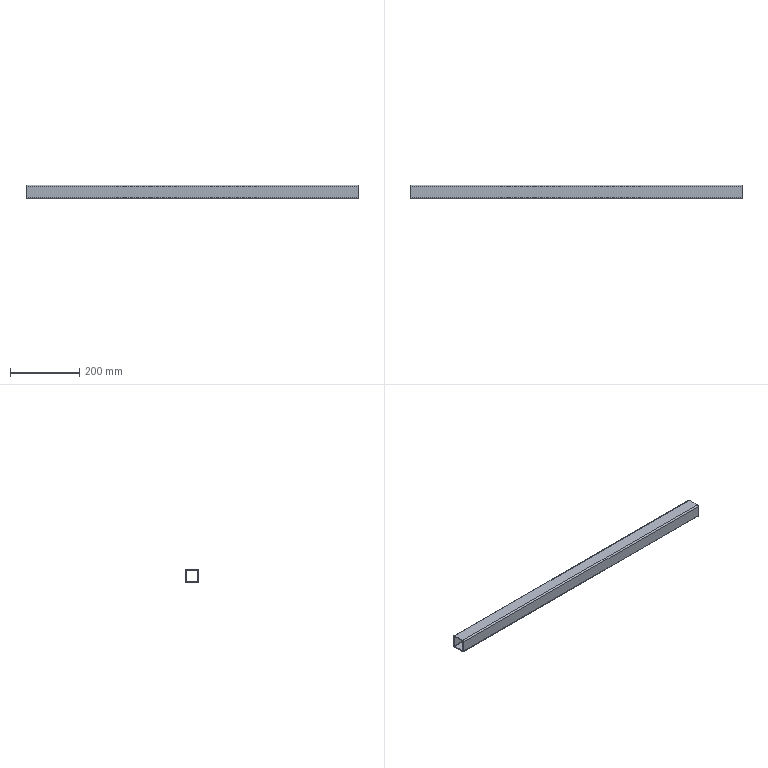Part | 1 solid | 22 faces | box 956 x 40 x 40 mm | volume 410269 mm3 | cylinder 12 | plane 10 | commonest cylinder face diameters 2 x4 8 x4 20 x4
STEP:
#1=CARTESIAN_POINT('',(40.,0.,-17.));
#2=VERTEX_POINT('',#1);
#3=CARTESIAN_POINT('',(60.,0.,-17.));
#4=VERTEX_POINT('',#3);
#5=CARTESIAN_POINT('',(50.,0.,-17.));
#6=DIRECTION('',(0.,0.,1.));
#7=DIRECTION('',(1.,0.,0.));
#8=AXIS2_PLACEMENT_3D('',#5,#6,#7);
#9=CIRCLE('',#8,10.);
#10=EDGE_CURVE('',#2,#4,#9,.T.);
#11=ORIENTED_EDGE('',*,*,#10,.T.);
#12=CARTESIAN_POINT('',(60.,0.,-20.));
#13=VERTEX_POINT('',#12);
#14=CARTESIAN_POINT('',(60.,0.,-10.));
#15=DIRECTION('',(0.,0.,-1.));
#16=VECTOR('',#15,1000.);
#17=LINE('',#14,#16);
#18=EDGE_CURVE('',#4,#13,#17,.T.);
#19=ORIENTED_EDGE('',*,*,#18,.T.);
#20=CARTESIAN_POINT('',(40.,0.,-20.));
#21=VERTEX_POINT('',#20);
#22=CARTESIAN_POINT('',(50.,0.,-20.));
#23=DIRECTION('',(0.,0.,-1.));
#24=DIRECTION('',(-1.,0.,0.));
#25=AXIS2_PLACEMENT_3D('',#22,#23,#24);
#26=CIRCLE('',#25,10.);
#27=EDGE_CURVE('',#13,#21,#26,.T.);
#28=ORIENTED_EDGE('',*,*,#27,.T.);
#29=CARTESIAN_POINT('',(40.,0.,-10.));
#30=DIRECTION('',(0.,0.,-1.));
#31=VECTOR('',#30,1000.);
#32=LINE('',#29,#31);
#33=EDGE_CURVE('',#2,#21,#32,.T.);
#34=ORIENTED_EDGE('',*,*,#33,.F.);
#35=EDGE_LOOP('',(#11,#19,#28,#34));
#36=FACE_OUTER_BOUND('',#35,.T.);
#37=CARTESIAN_POINT('',(50.,0.,-10.));
#38=DIRECTION('',(0.,0.,-1.));
#39=DIRECTION('',(-1.,0.,0.));
#40=AXIS2_PLACEMENT_3D('',#37,#38,#39);
#41=CYLINDRICAL_SURFACE('',#40,10.);
#42=ADVANCED_FACE('',(#36),#41,.F.);
#43=CARTESIAN_POINT('',(921.,0.,-17.));
#44=VERTEX_POINT('',#43);
#45=CARTESIAN_POINT('',(941.,0.,-17.));
#46=VERTEX_POINT('',#45);
#47=CARTESIAN_POINT('',(931.,0.,-17.));
#48=DIRECTION('',(0.,0.,1.));
#49=DIRECTION('',(1.,0.,0.));
#50=AXIS2_PLACEMENT_3D('',#47,#48,#49);
#51=CIRCLE('',#50,10.);
#52=EDGE_CURVE('',#44,#46,#51,.T.);
#53=ORIENTED_EDGE('',*,*,#52,.T.);
#54=CARTESIAN_POINT('',(941.,0.,-20.));
#55=VERTEX_POINT('',#54);
#56=CARTESIAN_POINT('',(941.,0.,-10.));
#57=DIRECTION('',(0.,0.,-1.));
#58=VECTOR('',#57,1000.);
#59=LINE('',#56,#58);
#60=EDGE_CURVE('',#46,#55,#59,.T.);
#61=ORIENTED_EDGE('',*,*,#60,.T.);
#62=CARTESIAN_POINT('',(921.,0.,-20.));
#63=VERTEX_POINT('',#62);
#64=CARTESIAN_POINT('',(931.,0.,-20.));
#65=DIRECTION('',(0.,0.,-1.));
#66=DIRECTION('',(-1.,0.,0.));
#67=AXIS2_PLACEMENT_3D('',#64,#65,#66);
#68=CIRCLE('',#67,10.);
#69=EDGE_CURVE('',#55,#63,#68,.T.);
#70=ORIENTED_EDGE('',*,*,#69,.T.);
#71=CARTESIAN_POINT('',(921.,0.,-10.));
#72=DIRECTION('',(0.,0.,-1.));
#73=VECTOR('',#72,1000.);
#74=LINE('',#71,#73);
#75=EDGE_CURVE('',#44,#63,#74,.T.);
#76=ORIENTED_EDGE('',*,*,#75,.F.);
#77=EDGE_LOOP('',(#53,#61,#70,#76));
#78=FACE_OUTER_BOUND('',#77,.T.);
#79=CARTESIAN_POINT('',(931.,0.,-10.));
#80=DIRECTION('',(0.,0.,-1.));
#81=DIRECTION('',(-1.,0.,0.));
#82=AXIS2_PLACEMENT_3D('',#79,#80,#81);
#83=CYLINDRICAL_SURFACE('',#82,10.);
#84=ADVANCED_FACE('',(#78),#83,.F.);
#85=CARTESIAN_POINT('',(0.,20.,16.));
#86=VERTEX_POINT('',#85);
#87=CARTESIAN_POINT('',(0.,16.,20.));
#88=VERTEX_POINT('',#87);
#89=CARTESIAN_POINT('',(0.,16.,16.));
#90=DIRECTION('',(1.,0.,0.));
#91=DIRECTION('',(0.,0.,-1.));
#92=AXIS2_PLACEMENT_3D('',#89,#90,#91);
#93=CIRCLE('',#92,4.);
#94=EDGE_CURVE('',#86,#88,#93,.T.);
#95=ORIENTED_EDGE('',*,*,#94,.T.);
#96=CARTESIAN_POINT('',(956.,16.,20.));
#97=VERTEX_POINT('',#96);
#98=CARTESIAN_POINT('',(956.,16.,20.));
#99=DIRECTION('',(-1.,0.,0.));
#100=VECTOR('',#99,1000.);
#101=LINE('',#98,#100);
#102=EDGE_CURVE('',#97,#88,#101,.T.);
#103=ORIENTED_EDGE('',*,*,#102,.F.);
#104=CARTESIAN_POINT('',(956.,20.,16.));
#105=VERTEX_POINT('',#104);
#106=CARTESIAN_POINT('',(956.,16.,16.));
#107=DIRECTION('',(1.,0.,0.));
#108=DIRECTION('',(0.,0.,-1.));
#109=AXIS2_PLACEMENT_3D('',#106,#107,#108);
#110=CIRCLE('',#109,4.);
#111=EDGE_CURVE('',#105,#97,#110,.T.);
#112=ORIENTED_EDGE('',*,*,#111,.F.);
#113=CARTESIAN_POINT('',(956.,20.,16.));
#114=DIRECTION('',(-1.,0.,0.));
#115=VECTOR('',#114,1000.);
#116=LINE('',#113,#115);
#117=EDGE_CURVE('',#105,#86,#116,.T.);
#118=ORIENTED_EDGE('',*,*,#117,.T.);
#119=EDGE_LOOP('',(#95,#103,#112,#118));
#120=FACE_OUTER_BOUND('',#119,.T.);
#121=CARTESIAN_POINT('',(956.,16.,16.));
#122=DIRECTION('',(-1.,0.,0.));
#123=DIRECTION('',(0.,0.,1.));
#124=AXIS2_PLACEMENT_3D('',#121,#122,#123);
#125=CYLINDRICAL_SURFACE('',#124,4.);
#126=ADVANCED_FACE('',(#120),#125,.T.);
#127=CARTESIAN_POINT('',(0.,-16.,20.));
#128=VERTEX_POINT('',#127);
#129=CARTESIAN_POINT('',(0.,16.,20.));
#130=DIRECTION('',(0.,-1.,0.));
#131=VECTOR('',#130,1000.);
#132=LINE('',#129,#131);
#133=EDGE_CURVE('',#88,#128,#132,.T.);
#134=ORIENTED_EDGE('',*,*,#133,.T.);
#135=CARTESIAN_POINT('',(956.,-16.,20.));
#136=VERTEX_POINT('',#135);
#137=CARTESIAN_POINT('',(956.,-16.,20.));
#138=DIRECTION('',(-1.,0.,0.));
#139=VECTOR('',#138,1000.);
#140=LINE('',#137,#139);
#141=EDGE_CURVE('',#136,#128,#140,.T.);
#142=ORIENTED_EDGE('',*,*,#141,.F.);
#143=CARTESIAN_POINT('',(956.,16.,20.));
#144=DIRECTION('',(0.,-1.,0.));
#145=VECTOR('',#144,1000.);
#146=LINE('',#143,#145);
#147=EDGE_CURVE('',#97,#136,#146,.T.);
#148=ORIENTED_EDGE('',*,*,#147,.F.);
#149=ORIENTED_EDGE('',*,*,#102,.T.);
#150=EDGE_LOOP('',(#134,#142,#148,#149));
#151=FACE_OUTER_BOUND('',#150,.T.);
#152=CARTESIAN_POINT('',(956.,16.,20.));
#153=DIRECTION('',(0.,0.,-1.));
#154=DIRECTION('',(-1.,0.,0.));
#155=AXIS2_PLACEMENT_3D('',#152,#153,#154);
#156=PLANE('',#155);
#157=ADVANCED_FACE('',(#151),#156,.F.);
#158=CARTESIAN_POINT('',(0.,-20.,16.));
#159=VERTEX_POINT('',#158);
#160=CARTESIAN_POINT('',(0.,-16.,16.));
#161=DIRECTION('',(1.,0.,0.));
#162=DIRECTION('',(0.,0.,-1.));
#163=AXIS2_PLACEMENT_3D('',#160,#161,#162);
#164=CIRCLE('',#163,4.);
#165=EDGE_CURVE('',#128,#159,#164,.T.);
#166=ORIENTED_EDGE('',*,*,#165,.T.);
#167=CARTESIAN_POINT('',(956.,-20.,16.));
#168=VERTEX_POINT('',#167);
#169=CARTESIAN_POINT('',(956.,-20.,16.));
#170=DIRECTION('',(-1.,0.,0.));
#171=VECTOR('',#170,1000.);
#172=LINE('',#169,#171);
#173=EDGE_CURVE('',#168,#159,#172,.T.);
#174=ORIENTED_EDGE('',*,*,#173,.F.);
#175=CARTESIAN_POINT('',(956.,-16.,16.));
#176=DIRECTION('',(1.,0.,0.));
#177=DIRECTION('',(0.,0.,-1.));
#178=AXIS2_PLACEMENT_3D('',#175,#176,#177);
#179=CIRCLE('',#178,4.);
#180=EDGE_CURVE('',#136,#168,#179,.T.);
#181=ORIENTED_EDGE('',*,*,#180,.F.);
#182=ORIENTED_EDGE('',*,*,#141,.T.);
#183=EDGE_LOOP('',(#166,#174,#181,#182));
#184=FACE_OUTER_BOUND('',#183,.T.);
#185=CARTESIAN_POINT('',(956.,-16.,16.));
#186=DIRECTION('',(-1.,0.,0.));
#187=DIRECTION('',(0.,0.,1.));
#188=AXIS2_PLACEMENT_3D('',#185,#186,#187);
#189=CYLINDRICAL_SURFACE('',#188,4.);
#190=ADVANCED_FACE('',(#184),#189,.T.);
#191=CARTESIAN_POINT('',(0.,-20.,-16.));
#192=VERTEX_POINT('',#191);
#193=CARTESIAN_POINT('',(0.,-20.,-16.));
#194=DIRECTION('',(0.,0.,-1.));
#195=VECTOR('',#194,1000.);
#196=LINE('',#193,#195);
#197=EDGE_CURVE('',#159,#192,#196,.T.);
#198=ORIENTED_EDGE('',*,*,#197,.T.);
#199=CARTESIAN_POINT('',(956.,-20.,-16.));
#200=VERTEX_POINT('',#199);
#201=CARTESIAN_POINT('',(956.,-20.,-16.));
#202=DIRECTION('',(-1.,0.,0.));
#203=VECTOR('',#202,1000.);
#204=LINE('',#201,#203);
#205=EDGE_CURVE('',#200,#192,#204,.T.);
#206=ORIENTED_EDGE('',*,*,#205,.F.);
#207=CARTESIAN_POINT('',(956.,-20.,-16.));
#208=DIRECTION('',(0.,0.,-1.));
#209=VECTOR('',#208,1000.);
#210=LINE('',#207,#209);
#211=EDGE_CURVE('',#168,#200,#210,.T.);
#212=ORIENTED_EDGE('',*,*,#211,.F.);
#213=ORIENTED_EDGE('',*,*,#173,.T.);
#214=EDGE_LOOP('',(#198,#206,#212,#213));
#215=FACE_OUTER_BOUND('',#214,.T.);
#216=CARTESIAN_POINT('',(956.,-20.,-16.));
#217=DIRECTION('',(0.,1.,0.));
#218=DIRECTION('',(0.,0.,1.));
#219=AXIS2_PLACEMENT_3D('',#216,#217,#218);
#220=PLANE('',#219);
#221=ADVANCED_FACE('',(#215),#220,.F.);
#222=CARTESIAN_POINT('',(0.,-16.,-20.));
#223=VERTEX_POINT('',#222);
#224=CARTESIAN_POINT('',(0.,-16.,-16.));
#225=DIRECTION('',(1.,0.,0.));
#226=DIRECTION('',(0.,0.,-1.));
#227=AXIS2_PLACEMENT_3D('',#224,#225,#226);
#228=CIRCLE('',#227,4.);
#229=EDGE_CURVE('',#192,#223,#228,.T.);
#230=ORIENTED_EDGE('',*,*,#229,.T.);
#231=CARTESIAN_POINT('',(956.,-16.,-20.));
#232=VERTEX_POINT('',#231);
#233=CARTESIAN_POINT('',(956.,-16.,-20.));
#234=DIRECTION('',(-1.,0.,0.));
#235=VECTOR('',#234,1000.);
#236=LINE('',#233,#235);
#237=EDGE_CURVE('',#232,#223,#236,.T.);
#238=ORIENTED_EDGE('',*,*,#237,.F.);
#239=CARTESIAN_POINT('',(956.,-16.,-16.));
#240=DIRECTION('',(1.,0.,0.));
#241=DIRECTION('',(0.,0.,-1.));
#242=AXIS2_PLACEMENT_3D('',#239,#240,#241);
#243=CIRCLE('',#242,4.);
#244=EDGE_CURVE('',#200,#232,#243,.T.);
#245=ORIENTED_EDGE('',*,*,#244,.F.);
#246=ORIENTED_EDGE('',*,*,#205,.T.);
#247=EDGE_LOOP('',(#230,#238,#245,#246));
#248=FACE_OUTER_BOUND('',#247,.T.);
#249=CARTESIAN_POINT('',(956.,-16.,-16.));
#250=DIRECTION('',(-1.,0.,0.));
#251=DIRECTION('',(0.,0.,1.));
#252=AXIS2_PLACEMENT_3D('',#249,#250,#251);
#253=CYLINDRICAL_SURFACE('',#252,4.);
#254=ADVANCED_FACE('',(#248),#253,.T.);
#255=CARTESIAN_POINT('',(50.,0.,-20.));
#256=DIRECTION('',(0.,0.,-1.));
#257=DIRECTION('',(-1.,0.,0.));
#258=AXIS2_PLACEMENT_3D('',#255,#256,#257);
#259=CIRCLE('',#258,10.);
#260=EDGE_CURVE('',#21,#13,#259,.T.);
#261=ORIENTED_EDGE('',*,*,#260,.F.);
#262=ORIENTED_EDGE('',*,*,#27,.F.);
#263=EDGE_LOOP('',(#261,#262));
#264=FACE_BOUND('',#263,.T.);
#265=CARTESIAN_POINT('',(931.,0.,-20.));
#266=DIRECTION('',(0.,0.,-1.));
#267=DIRECTION('',(-1.,0.,0.));
#268=AXIS2_PLACEMENT_3D('',#265,#266,#267);
#269=CIRCLE('',#268,10.);
#270=EDGE_CURVE('',#63,#55,#269,.T.);
#271=ORIENTED_EDGE('',*,*,#270,.F.);
#272=ORIENTED_EDGE('',*,*,#69,.F.);
#273=EDGE_LOOP('',(#271,#272));
#274=FACE_BOUND('',#273,.T.);
#275=CARTESIAN_POINT('',(0.,16.,-20.));
#276=VERTEX_POINT('',#275);
#277=CARTESIAN_POINT('',(0.,-16.,-20.));
#278=DIRECTION('',(0.,1.,0.));
#279=VECTOR('',#278,1000.);
#280=LINE('',#277,#279);
#281=EDGE_CURVE('',#223,#276,#280,.T.);
#282=ORIENTED_EDGE('',*,*,#281,.T.);
#283=CARTESIAN_POINT('',(956.,16.,-20.));
#284=VERTEX_POINT('',#283);
#285=CARTESIAN_POINT('',(956.,16.,-20.));
#286=DIRECTION('',(-1.,0.,0.));
#287=VECTOR('',#286,1000.);
#288=LINE('',#285,#287);
#289=EDGE_CURVE('',#284,#276,#288,.T.);
#290=ORIENTED_EDGE('',*,*,#289,.F.);
#291=CARTESIAN_POINT('',(956.,-16.,-20.));
#292=DIRECTION('',(0.,1.,0.));
#293=VECTOR('',#292,1000.);
#294=LINE('',#291,#293);
#295=EDGE_CURVE('',#232,#284,#294,.T.);
#296=ORIENTED_EDGE('',*,*,#295,.F.);
#297=ORIENTED_EDGE('',*,*,#237,.T.);
#298=EDGE_LOOP('',(#282,#290,#296,#297));
#299=FACE_OUTER_BOUND('',#298,.T.);
#300=CARTESIAN_POINT('',(956.,-16.,-20.));
#301=DIRECTION('',(0.,0.,1.));
#302=DIRECTION('',(1.,0.,0.));
#303=AXIS2_PLACEMENT_3D('',#300,#301,#302);
#304=PLANE('',#303);
#305=ADVANCED_FACE('',(#264,#274,#299),#304,.F.);
#306=CARTESIAN_POINT('',(0.,20.,-16.));
#307=VERTEX_POINT('',#306);
#308=CARTESIAN_POINT('',(0.,16.,-16.));
#309=DIRECTION('',(1.,0.,0.));
#310=DIRECTION('',(0.,0.,-1.));
#311=AXIS2_PLACEMENT_3D('',#308,#309,#310);
#312=CIRCLE('',#311,4.);
#313=EDGE_CURVE('',#276,#307,#312,.T.);
#314=ORIENTED_EDGE('',*,*,#313,.T.);
#315=CARTESIAN_POINT('',(956.,20.,-16.));
#316=VERTEX_POINT('',#315);
#317=CARTESIAN_POINT('',(956.,20.,-16.));
#318=DIRECTION('',(-1.,0.,0.));
#319=VECTOR('',#318,1000.);
#320=LINE('',#317,#319);
#321=EDGE_CURVE('',#316,#307,#320,.T.);
#322=ORIENTED_EDGE('',*,*,#321,.F.);
#323=CARTESIAN_POINT('',(956.,16.,-16.));
#324=DIRECTION('',(1.,0.,0.));
#325=DIRECTION('',(0.,0.,-1.));
#326=AXIS2_PLACEMENT_3D('',#323,#324,#325);
#327=CIRCLE('',#326,4.);
#328=EDGE_CURVE('',#284,#316,#327,.T.);
#329=ORIENTED_EDGE('',*,*,#328,.F.);
#330=ORIENTED_EDGE('',*,*,#289,.T.);
#331=EDGE_LOOP('',(#314,#322,#329,#330));
#332=FACE_OUTER_BOUND('',#331,.T.);
#333=CARTESIAN_POINT('',(956.,16.,-16.));
#334=DIRECTION('',(-1.,0.,0.));
#335=DIRECTION('',(0.,0.,1.));
#336=AXIS2_PLACEMENT_3D('',#333,#334,#335);
#337=CYLINDRICAL_SURFACE('',#336,4.);
#338=ADVANCED_FACE('',(#332),#337,.T.);
#339=CARTESIAN_POINT('',(0.,-16.,17.));
#340=VERTEX_POINT('',#339);
#341=CARTESIAN_POINT('',(0.,-17.,16.));
#342=VERTEX_POINT('',#341);
#343=CARTESIAN_POINT('',(0.,-16.,16.));
#344=DIRECTION('',(1.,0.,0.));
#345=DIRECTION('',(0.,0.,-1.));
#346=AXIS2_PLACEMENT_3D('',#343,#344,#345);
#347=CIRCLE('',#346,1.);
#348=EDGE_CURVE('',#340,#342,#347,.T.);
#349=ORIENTED_EDGE('',*,*,#348,.F.);
#350=CARTESIAN_POINT('',(956.,-16.,17.));
#351=VERTEX_POINT('',#350);
#352=CARTESIAN_POINT('',(956.,-16.,17.));
#353=DIRECTION('',(-1.,0.,0.));
#354=VECTOR('',#353,1000.);
#355=LINE('',#352,#354);
#356=EDGE_CURVE('',#351,#340,#355,.T.);
#357=ORIENTED_EDGE('',*,*,#356,.F.);
#358=CARTESIAN_POINT('',(956.,-17.,16.));
#359=VERTEX_POINT('',#358);
#360=CARTESIAN_POINT('',(956.,-16.,16.));
#361=DIRECTION('',(1.,0.,0.));
#362=DIRECTION('',(0.,0.,-1.));
#363=AXIS2_PLACEMENT_3D('',#360,#361,#362);
#364=CIRCLE('',#363,1.);
#365=EDGE_CURVE('',#351,#359,#364,.T.);
#366=ORIENTED_EDGE('',*,*,#365,.T.);
#367=CARTESIAN_POINT('',(956.,-17.,16.));
#368=DIRECTION('',(-1.,0.,0.));
#369=VECTOR('',#368,1000.);
#370=LINE('',#367,#369);
#371=EDGE_CURVE('',#359,#342,#370,.T.);
#372=ORIENTED_EDGE('',*,*,#371,.T.);
#373=EDGE_LOOP('',(#349,#357,#366,#372));
#374=FACE_OUTER_BOUND('',#373,.T.);
#375=CARTESIAN_POINT('',(956.,-16.,16.));
#376=DIRECTION('',(-1.,0.,0.));
#377=DIRECTION('',(0.,0.,1.));
#378=AXIS2_PLACEMENT_3D('',#375,#376,#377);
#379=CYLINDRICAL_SURFACE('',#378,1.);
#380=ADVANCED_FACE('',(#374),#379,.F.);
#381=CARTESIAN_POINT('',(0.,16.,17.));
#382=VERTEX_POINT('',#381);
#383=CARTESIAN_POINT('',(0.,16.,17.));
#384=DIRECTION('',(0.,-1.,0.));
#385=VECTOR('',#384,1000.);
#386=LINE('',#383,#385);
#387=EDGE_CURVE('',#382,#340,#386,.T.);
#388=ORIENTED_EDGE('',*,*,#387,.F.);
#389=CARTESIAN_POINT('',(956.,16.,17.));
#390=VERTEX_POINT('',#389);
#391=CARTESIAN_POINT('',(956.,16.,17.));
#392=DIRECTION('',(-1.,0.,0.));
#393=VECTOR('',#392,1000.);
#394=LINE('',#391,#393);
#395=EDGE_CURVE('',#390,#382,#394,.T.);
#396=ORIENTED_EDGE('',*,*,#395,.F.);
#397=CARTESIAN_POINT('',(956.,16.,17.));
#398=DIRECTION('',(0.,-1.,0.));
#399=VECTOR('',#398,1000.);
#400=LINE('',#397,#399);
#401=EDGE_CURVE('',#390,#351,#400,.T.);
#402=ORIENTED_EDGE('',*,*,#401,.T.);
#403=ORIENTED_EDGE('',*,*,#356,.T.);
#404=EDGE_LOOP('',(#388,#396,#402,#403));
#405=FACE_OUTER_BOUND('',#404,.T.);
#406=CARTESIAN_POINT('',(956.,16.,17.));
#407=DIRECTION('',(0.,0.,-1.));
#408=DIRECTION('',(-1.,0.,0.));
#409=AXIS2_PLACEMENT_3D('',#406,#407,#408);
#410=PLANE('',#409);
#411=ADVANCED_FACE('',(#405),#410,.T.);
#412=CARTESIAN_POINT('',(0.,17.,16.));
#413=VERTEX_POINT('',#412);
#414=CARTESIAN_POINT('',(0.,16.,16.));
#415=DIRECTION('',(1.,0.,0.));
#416=DIRECTION('',(0.,0.,-1.));
#417=AXIS2_PLACEMENT_3D('',#414,#415,#416);
#418=CIRCLE('',#417,1.);
#419=EDGE_CURVE('',#413,#382,#418,.T.);
#420=ORIENTED_EDGE('',*,*,#419,.F.);
#421=CARTESIAN_POINT('',(956.,17.,16.));
#422=VERTEX_POINT('',#421);
#423=CARTESIAN_POINT('',(956.,17.,16.));
#424=DIRECTION('',(-1.,0.,0.));
#425=VECTOR('',#424,1000.);
#426=LINE('',#423,#425);
#427=EDGE_CURVE('',#422,#413,#426,.T.);
#428=ORIENTED_EDGE('',*,*,#427,.F.);
#429=CARTESIAN_POINT('',(956.,16.,16.));
#430=DIRECTION('',(1.,0.,0.));
#431=DIRECTION('',(0.,0.,-1.));
#432=AXIS2_PLACEMENT_3D('',#429,#430,#431);
#433=CIRCLE('',#432,1.);
#434=EDGE_CURVE('',#422,#390,#433,.T.);
#435=ORIENTED_EDGE('',*,*,#434,.T.);
#436=ORIENTED_EDGE('',*,*,#395,.T.);
#437=EDGE_LOOP('',(#420,#428,#435,#436));
#438=FACE_OUTER_BOUND('',#437,.T.);
#439=CARTESIAN_POINT('',(956.,16.,16.));
#440=DIRECTION('',(-1.,0.,0.));
#441=DIRECTION('',(0.,0.,1.));
#442=AXIS2_PLACEMENT_3D('',#439,#440,#441);
#443=CYLINDRICAL_SURFACE('',#442,1.);
#444=ADVANCED_FACE('',(#438),#443,.F.);
#445=CARTESIAN_POINT('',(0.,17.,-16.));
#446=VERTEX_POINT('',#445);
#447=CARTESIAN_POINT('',(0.,17.,16.));
#448=DIRECTION('',(0.,0.,1.));
#449=VECTOR('',#448,1000.);
#450=LINE('',#447,#449);
#451=EDGE_CURVE('',#446,#413,#450,.T.);
#452=ORIENTED_EDGE('',*,*,#451,.F.);
#453=CARTESIAN_POINT('',(956.,17.,-16.));
#454=VERTEX_POINT('',#453);
#455=CARTESIAN_POINT('',(956.,17.,-16.));
#456=DIRECTION('',(-1.,0.,0.));
#457=VECTOR('',#456,1000.);
#458=LINE('',#455,#457);
#459=EDGE_CURVE('',#454,#446,#458,.T.);
#460=ORIENTED_EDGE('',*,*,#459,.F.);
#461=CARTESIAN_POINT('',(956.,17.,16.));
#462=DIRECTION('',(0.,0.,1.));
#463=VECTOR('',#462,1000.);
#464=LINE('',#461,#463);
#465=EDGE_CURVE('',#454,#422,#464,.T.);
#466=ORIENTED_EDGE('',*,*,#465,.T.);
#467=ORIENTED_EDGE('',*,*,#427,.T.);
#468=EDGE_LOOP('',(#452,#460,#466,#467));
#469=FACE_OUTER_BOUND('',#468,.T.);
#470=CARTESIAN_POINT('',(956.,17.,16.));
#471=DIRECTION('',(0.,-1.,0.));
#472=DIRECTION('',(0.,0.,-1.));
#473=AXIS2_PLACEMENT_3D('',#470,#471,#472);
#474=PLANE('',#473);
#475=ADVANCED_FACE('',(#469),#474,.T.);
#476=CARTESIAN_POINT('',(0.,16.,-17.));
#477=VERTEX_POINT('',#476);
#478=CARTESIAN_POINT('',(0.,16.,-16.));
#479=DIRECTION('',(1.,0.,0.));
#480=DIRECTION('',(0.,0.,-1.));
#481=AXIS2_PLACEMENT_3D('',#478,#479,#480);
#482=CIRCLE('',#481,1.);
#483=EDGE_CURVE('',#477,#446,#482,.T.);
#484=ORIENTED_EDGE('',*,*,#483,.F.);
#485=CARTESIAN_POINT('',(956.,16.,-17.));
#486=VERTEX_POINT('',#485);
#487=CARTESIAN_POINT('',(956.,16.,-17.));
#488=DIRECTION('',(-1.,0.,0.));
#489=VECTOR('',#488,1000.);
#490=LINE('',#487,#489);
#491=EDGE_CURVE('',#486,#477,#490,.T.);
#492=ORIENTED_EDGE('',*,*,#491,.F.);
#493=CARTESIAN_POINT('',(956.,16.,-16.));
#494=DIRECTION('',(1.,0.,0.));
#495=DIRECTION('',(0.,0.,-1.));
#496=AXIS2_PLACEMENT_3D('',#493,#494,#495);
#497=CIRCLE('',#496,1.);
#498=EDGE_CURVE('',#486,#454,#497,.T.);
#499=ORIENTED_EDGE('',*,*,#498,.T.);
#500=ORIENTED_EDGE('',*,*,#459,.T.);
#501=EDGE_LOOP('',(#484,#492,#499,#500));
#502=FACE_OUTER_BOUND('',#501,.T.);
#503=CARTESIAN_POINT('',(956.,16.,-16.));
#504=DIRECTION('',(-1.,0.,0.));
#505=DIRECTION('',(0.,0.,1.));
#506=AXIS2_PLACEMENT_3D('',#503,#504,#505);
#507=CYLINDRICAL_SURFACE('',#506,1.);
#508=ADVANCED_FACE('',(#502),#507,.F.);
#509=ORIENTED_EDGE('',*,*,#10,.F.);
#510=CARTESIAN_POINT('',(50.,0.,-17.));
#511=DIRECTION('',(0.,0.,1.));
#512=DIRECTION('',(1.,0.,0.));
#513=AXIS2_PLACEMENT_3D('',#510,#511,#512);
#514=CIRCLE('',#513,10.);
#515=EDGE_CURVE('',#4,#2,#514,.T.);
#516=ORIENTED_EDGE('',*,*,#515,.F.);
#517=EDGE_LOOP('',(#509,#516));
#518=FACE_BOUND('',#517,.T.);
#519=ORIENTED_EDGE('',*,*,#52,.F.);
#520=CARTESIAN_POINT('',(931.,0.,-17.));
#521=DIRECTION('',(0.,0.,1.));
#522=DIRECTION('',(1.,0.,0.));
#523=AXIS2_PLACEMENT_3D('',#520,#521,#522);
#524=CIRCLE('',#523,10.);
#525=EDGE_CURVE('',#46,#44,#524,.T.);
#526=ORIENTED_EDGE('',*,*,#525,.F.);
#527=EDGE_LOOP('',(#519,#526));
#528=FACE_BOUND('',#527,.T.);
#529=CARTESIAN_POINT('',(0.,-16.,-17.));
#530=VERTEX_POINT('',#529);
#531=CARTESIAN_POINT('',(0.,-16.,-17.));
#532=DIRECTION('',(0.,1.,0.));
#533=VECTOR('',#532,1000.);
#534=LINE('',#531,#533);
#535=EDGE_CURVE('',#530,#477,#534,.T.);
#536=ORIENTED_EDGE('',*,*,#535,.F.);
#537=CARTESIAN_POINT('',(956.,-16.,-17.));
#538=VERTEX_POINT('',#537);
#539=CARTESIAN_POINT('',(956.,-16.,-17.));
#540=DIRECTION('',(-1.,0.,0.));
#541=VECTOR('',#540,1000.);
#542=LINE('',#539,#541);
#543=EDGE_CURVE('',#538,#530,#542,.T.);
#544=ORIENTED_EDGE('',*,*,#543,.F.);
#545=CARTESIAN_POINT('',(956.,-16.,-17.));
#546=DIRECTION('',(0.,1.,0.));
#547=VECTOR('',#546,1000.);
#548=LINE('',#545,#547);
#549=EDGE_CURVE('',#538,#486,#548,.T.);
#550=ORIENTED_EDGE('',*,*,#549,.T.);
#551=ORIENTED_EDGE('',*,*,#491,.T.);
#552=EDGE_LOOP('',(#536,#544,#550,#551));
#553=FACE_OUTER_BOUND('',#552,.T.);
#554=CARTESIAN_POINT('',(956.,-16.,-17.));
#555=DIRECTION('',(0.,0.,1.));
#556=DIRECTION('',(1.,0.,0.));
#557=AXIS2_PLACEMENT_3D('',#554,#555,#556);
#558=PLANE('',#557);
#559=ADVANCED_FACE('',(#518,#528,#553),#558,.T.);
#560=CARTESIAN_POINT('',(0.,-17.,-16.));
#561=VERTEX_POINT('',#560);
#562=CARTESIAN_POINT('',(0.,-16.,-16.));
#563=DIRECTION('',(1.,0.,0.));
#564=DIRECTION('',(0.,0.,-1.));
#565=AXIS2_PLACEMENT_3D('',#562,#563,#564);
#566=CIRCLE('',#565,1.);
#567=EDGE_CURVE('',#561,#530,#566,.T.);
#568=ORIENTED_EDGE('',*,*,#567,.F.);
#569=CARTESIAN_POINT('',(956.,-17.,-16.));
#570=VERTEX_POINT('',#569);
#571=CARTESIAN_POINT('',(956.,-17.,-16.));
#572=DIRECTION('',(-1.,0.,0.));
#573=VECTOR('',#572,1000.);
#574=LINE('',#571,#573);
#575=EDGE_CURVE('',#570,#561,#574,.T.);
#576=ORIENTED_EDGE('',*,*,#575,.F.);
#577=CARTESIAN_POINT('',(956.,-16.,-16.));
#578=DIRECTION('',(1.,0.,0.));
#579=DIRECTION('',(0.,0.,-1.));
#580=AXIS2_PLACEMENT_3D('',#577,#578,#579);
#581=CIRCLE('',#580,1.);
#582=EDGE_CURVE('',#570,#538,#581,.T.);
#583=ORIENTED_EDGE('',*,*,#582,.T.);
#584=ORIENTED_EDGE('',*,*,#543,.T.);
#585=EDGE_LOOP('',(#568,#576,#583,#584));
#586=FACE_OUTER_BOUND('',#585,.T.);
#587=CARTESIAN_POINT('',(956.,-16.,-16.));
#588=DIRECTION('',(-1.,0.,0.));
#589=DIRECTION('',(0.,0.,1.));
#590=AXIS2_PLACEMENT_3D('',#587,#588,#589);
#591=CYLINDRICAL_SURFACE('',#590,1.);
#592=ADVANCED_FACE('',(#586),#591,.F.);
#593=CARTESIAN_POINT('',(0.,-17.,-16.));
#594=DIRECTION('',(0.,0.,-1.));
#595=VECTOR('',#594,1000.);
#596=LINE('',#593,#595);
#597=EDGE_CURVE('',#342,#561,#596,.T.);
#598=ORIENTED_EDGE('',*,*,#597,.F.);
#599=ORIENTED_EDGE('',*,*,#371,.F.);
#600=CARTESIAN_POINT('',(956.,-17.,-16.));
#601=DIRECTION('',(0.,0.,-1.));
#602=VECTOR('',#601,1000.);
#603=LINE('',#600,#602);
#604=EDGE_CURVE('',#359,#570,#603,.T.);
#605=ORIENTED_EDGE('',*,*,#604,.T.);
#606=ORIENTED_EDGE('',*,*,#575,.T.);
#607=EDGE_LOOP('',(#598,#599,#605,#606));
#608=FACE_OUTER_BOUND('',#607,.T.);
#609=CARTESIAN_POINT('',(956.,-17.,-16.));
#610=DIRECTION('',(0.,1.,0.));
#611=DIRECTION('',(0.,0.,1.));
#612=AXIS2_PLACEMENT_3D('',#609,#610,#611);
#613=PLANE('',#612);
#614=ADVANCED_FACE('',(#608),#613,.T.);
#615=CARTESIAN_POINT('',(0.,20.,16.));
#616=DIRECTION('',(0.,0.,1.));
#617=VECTOR('',#616,1000.);
#618=LINE('',#615,#617);
#619=EDGE_CURVE('',#307,#86,#618,.T.);
#620=ORIENTED_EDGE('',*,*,#619,.T.);
#621=ORIENTED_EDGE('',*,*,#117,.F.);
#622=CARTESIAN_POINT('',(956.,20.,16.));
#623=DIRECTION('',(0.,0.,1.));
#624=VECTOR('',#623,1000.);
#625=LINE('',#622,#624);
#626=EDGE_CURVE('',#316,#105,#625,.T.);
#627=ORIENTED_EDGE('',*,*,#626,.F.);
#628=ORIENTED_EDGE('',*,*,#321,.T.);
#629=EDGE_LOOP('',(#620,#621,#627,#628));
#630=FACE_OUTER_BOUND('',#629,.T.);
#631=CARTESIAN_POINT('',(956.,20.,16.));
#632=DIRECTION('',(0.,-1.,0.));
#633=DIRECTION('',(0.,0.,-1.));
#634=AXIS2_PLACEMENT_3D('',#631,#632,#633);
#635=PLANE('',#634);
#636=ADVANCED_FACE('',(#630),#635,.F.);
#637=ORIENTED_EDGE('',*,*,#365,.F.);
#638=ORIENTED_EDGE('',*,*,#401,.F.);
#639=ORIENTED_EDGE('',*,*,#434,.F.);
#640=ORIENTED_EDGE('',*,*,#465,.F.);
#641=ORIENTED_EDGE('',*,*,#498,.F.);
#642=ORIENTED_EDGE('',*,*,#549,.F.);
#643=ORIENTED_EDGE('',*,*,#582,.F.);
#644=ORIENTED_EDGE('',*,*,#604,.F.);
#645=EDGE_LOOP('',(#637,#638,#639,#640,#641,#642,#643,#644));
#646=FACE_BOUND('',#645,.T.);
#647=ORIENTED_EDGE('',*,*,#111,.T.);
#648=ORIENTED_EDGE('',*,*,#147,.T.);
#649=ORIENTED_EDGE('',*,*,#180,.T.);
#650=ORIENTED_EDGE('',*,*,#211,.T.);
#651=ORIENTED_EDGE('',*,*,#244,.T.);
#652=ORIENTED_EDGE('',*,*,#295,.T.);
#653=ORIENTED_EDGE('',*,*,#328,.T.);
#654=ORIENTED_EDGE('',*,*,#626,.T.);
#655=EDGE_LOOP('',(#647,#648,#649,#650,#651,#652,#653,#654));
#656=FACE_OUTER_BOUND('',#655,.T.);
#657=CARTESIAN_POINT('',(956.,16.,16.));
#658=DIRECTION('',(1.,0.,0.));
#659=DIRECTION('',(0.,0.,-1.));
#660=AXIS2_PLACEMENT_3D('',#657,#658,#659);
#661=PLANE('',#660);
#662=ADVANCED_FACE('',(#646,#656),#661,.T.);
#663=ORIENTED_EDGE('',*,*,#348,.T.);
#664=ORIENTED_EDGE('',*,*,#597,.T.);
#665=ORIENTED_EDGE('',*,*,#567,.T.);
#666=ORIENTED_EDGE('',*,*,#535,.T.);
#667=ORIENTED_EDGE('',*,*,#483,.T.);
#668=ORIENTED_EDGE('',*,*,#451,.T.);
#669=ORIENTED_EDGE('',*,*,#419,.T.);
#670=ORIENTED_EDGE('',*,*,#387,.T.);
#671=EDGE_LOOP('',(#663,#664,#665,#666,#667,#668,#669,#670));
#672=FACE_BOUND('',#671,.T.);
#673=ORIENTED_EDGE('',*,*,#94,.F.);
#674=ORIENTED_EDGE('',*,*,#619,.F.);
#675=ORIENTED_EDGE('',*,*,#313,.F.);
#676=ORIENTED_EDGE('',*,*,#281,.F.);
#677=ORIENTED_EDGE('',*,*,#229,.F.);
#678=ORIENTED_EDGE('',*,*,#197,.F.);
#679=ORIENTED_EDGE('',*,*,#165,.F.);
#680=ORIENTED_EDGE('',*,*,#133,.F.);
#681=EDGE_LOOP('',(#673,#674,#675,#676,#677,#678,#679,#680));
#682=FACE_OUTER_BOUND('',#681,.T.);
#683=CARTESIAN_POINT('',(0.,16.,16.));
#684=DIRECTION('',(1.,0.,0.));
#685=DIRECTION('',(0.,0.,-1.));
#686=AXIS2_PLACEMENT_3D('',#683,#684,#685);
#687=PLANE('',#686);
#688=ADVANCED_FACE('',(#672,#682),#687,.F.);
#689=ORIENTED_EDGE('',*,*,#60,.F.);
#690=ORIENTED_EDGE('',*,*,#525,.T.);
#691=ORIENTED_EDGE('',*,*,#75,.T.);
#692=ORIENTED_EDGE('',*,*,#270,.T.);
#693=EDGE_LOOP('',(#689,#690,#691,#692));
#694=FACE_OUTER_BOUND('',#693,.T.);
#695=CARTESIAN_POINT('',(931.,0.,-10.));
#696=DIRECTION('',(0.,0.,-1.));
#697=DIRECTION('',(-1.,0.,0.));
#698=AXIS2_PLACEMENT_3D('',#695,#696,#697);
#699=CYLINDRICAL_SURFACE('',#698,10.);
#700=ADVANCED_FACE('',(#694),#699,.F.);
#701=ORIENTED_EDGE('',*,*,#18,.F.);
#702=ORIENTED_EDGE('',*,*,#515,.T.);
#703=ORIENTED_EDGE('',*,*,#33,.T.);
#704=ORIENTED_EDGE('',*,*,#260,.T.);
#705=EDGE_LOOP('',(#701,#702,#703,#704));
#706=FACE_OUTER_BOUND('',#705,.T.);
#707=CARTESIAN_POINT('',(50.,0.,-10.));
#708=DIRECTION('',(0.,0.,-1.));
#709=DIRECTION('',(-1.,0.,0.));
#710=AXIS2_PLACEMENT_3D('',#707,#708,#709);
#711=CYLINDRICAL_SURFACE('',#710,10.);
#712=ADVANCED_FACE('',(#706),#711,.F.);
#713=CLOSED_SHELL('',(#42,#84,#126,#157,#190,#221,#254,#305,#338,#380,#411,#444,#475,#508,#559,#592,#614,#636,#662,#688,#700,#712));
#714=MANIFOLD_SOLID_BREP('',#713);
#715=CARTESIAN_POINT('',(0.,0.,0.));
#716=DIRECTION('',(0.,0.,1.));
#717=DIRECTION('',(1.,0.,0.));
#718=AXIS2_PLACEMENT_3D('',#715,#716,#717);
#719=(LENGTH_UNIT()NAMED_UNIT(*)SI_UNIT(.MILLI.,.METRE.));
#720=UNCERTAINTY_MEASURE_WITH_UNIT(LENGTH_MEASURE(0.00001),#719,'','');
#721=(NAMED_UNIT(*)PLANE_ANGLE_UNIT()SI_UNIT($,.RADIAN.));
#722=(NAMED_UNIT(*)SI_UNIT($,.STERADIAN.)SOLID_ANGLE_UNIT());
#723=(GEOMETRIC_REPRESENTATION_CONTEXT(3)GLOBAL_UNCERTAINTY_ASSIGNED_CONTEXT((#720))GLOBAL_UNIT_ASSIGNED_CONTEXT((#719,#721,#722))REPRESENTATION_CONTEXT('',''));
#724=ADVANCED_BREP_SHAPE_REPRESENTATION('',(#714,#718),#723);